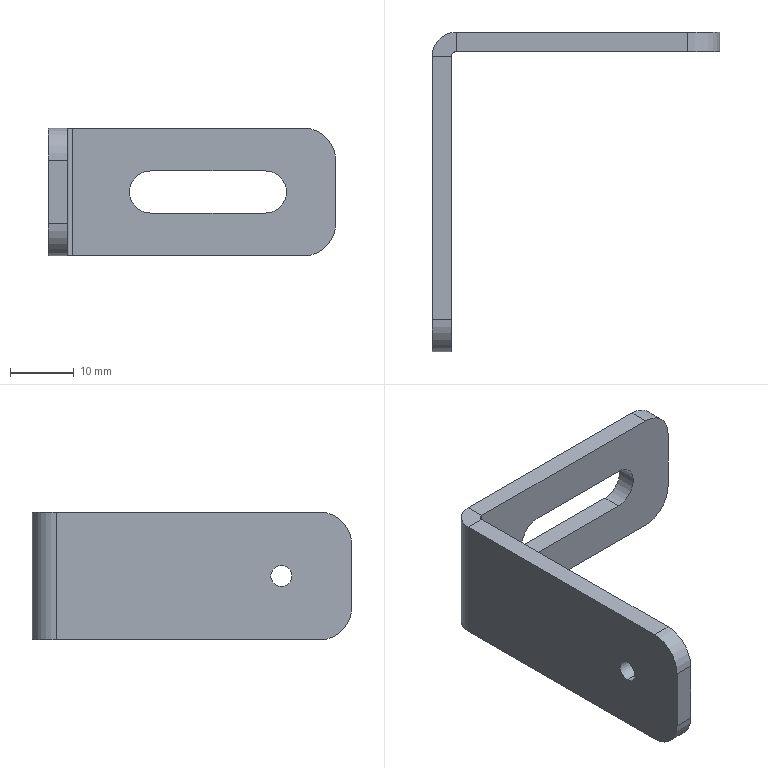Part | SolidWorks | features 3DProfileFeature 1, Fillet 1, FlatPattern 1, HoleWzd 1, ICE 1, SMBaseFlange 1, SheetMetal 1 | 1 solid | 24 faces | box 45 x 50 x 20 mm | volume 4913 mm3 | plane 14 | cylinder 10 | commonest cylinder face diameters 10 x4 3.3 x2 6.6 x2 1.473 x1 7.473 x1
STEP:
#1=CARTESIAN_POINT('',(0.,-39.,11.65));
#2=VERTEX_POINT('',#1);
#3=CARTESIAN_POINT('',(0.,-39.,8.35));
#4=VERTEX_POINT('',#3);
#5=CARTESIAN_POINT('',(0.,-39.,10.));
#6=DIRECTION('',(1.,0.,0.));
#7=DIRECTION('',(0.,0.,-1.));
#8=AXIS2_PLACEMENT_3D('',#5,#6,#7);
#9=CIRCLE('',#8,1.65);
#10=EDGE_CURVE('',#2,#4,#9,.T.);
#11=ORIENTED_EDGE('',*,*,#10,.F.);
#12=CARTESIAN_POINT('',(3.,-39.,11.65));
#13=VERTEX_POINT('',#12);
#14=CARTESIAN_POINT('',(3.,-39.,11.65));
#15=DIRECTION('',(1.,0.,0.));
#16=VECTOR('',#15,1000.);
#17=LINE('',#14,#16);
#18=EDGE_CURVE('',#2,#13,#17,.T.);
#19=ORIENTED_EDGE('',*,*,#18,.T.);
#20=CARTESIAN_POINT('',(3.,-39.,8.35));
#21=VERTEX_POINT('',#20);
#22=CARTESIAN_POINT('',(3.,-39.,10.));
#23=DIRECTION('',(1.,0.,0.));
#24=DIRECTION('',(0.,0.,-1.));
#25=AXIS2_PLACEMENT_3D('',#22,#23,#24);
#26=CIRCLE('',#25,1.65);
#27=EDGE_CURVE('',#13,#21,#26,.T.);
#28=ORIENTED_EDGE('',*,*,#27,.T.);
#29=CARTESIAN_POINT('',(3.,-39.,8.35));
#30=DIRECTION('',(1.,0.,0.));
#31=VECTOR('',#30,1000.);
#32=LINE('',#29,#31);
#33=EDGE_CURVE('',#4,#21,#32,.T.);
#34=ORIENTED_EDGE('',*,*,#33,.F.);
#35=EDGE_LOOP('',(#11,#19,#28,#34));
#36=FACE_OUTER_BOUND('',#35,.T.);
#37=CARTESIAN_POINT('',(3.,-39.,10.));
#38=DIRECTION('',(1.,0.,0.));
#39=DIRECTION('',(0.,0.,-1.));
#40=AXIS2_PLACEMENT_3D('',#37,#38,#39);
#41=CYLINDRICAL_SURFACE('',#40,1.65);
#42=ADVANCED_FACE('',(#36),#41,.F.);
#43=CARTESIAN_POINT('',(3.737,0.,20.));
#44=VERTEX_POINT('',#43);
#45=CARTESIAN_POINT('',(3.737,-3.,20.));
#46=VERTEX_POINT('',#45);
#47=CARTESIAN_POINT('',(3.737,0.,20.));
#48=DIRECTION('',(0.,-1.,0.));
#49=VECTOR('',#48,1000.);
#50=LINE('',#47,#49);
#51=EDGE_CURVE('',#44,#46,#50,.T.);
#52=ORIENTED_EDGE('',*,*,#51,.F.);
#53=CARTESIAN_POINT('',(0.,-3.737,20.));
#54=VERTEX_POINT('',#53);
#55=CARTESIAN_POINT('',(3.737,-3.737,20.));
#56=DIRECTION('',(0.,0.,-1.));
#57=DIRECTION('',(1.,0.,0.));
#58=AXIS2_PLACEMENT_3D('',#55,#56,#57);
#59=CIRCLE('',#58,3.737);
#60=EDGE_CURVE('',#54,#44,#59,.T.);
#61=ORIENTED_EDGE('',*,*,#60,.F.);
#62=CARTESIAN_POINT('',(3.,-3.737,20.));
#63=VERTEX_POINT('',#62);
#64=CARTESIAN_POINT('',(3.,-3.737,20.));
#65=DIRECTION('',(-1.,0.,0.));
#66=VECTOR('',#65,1000.);
#67=LINE('',#64,#66);
#68=EDGE_CURVE('',#63,#54,#67,.T.);
#69=ORIENTED_EDGE('',*,*,#68,.F.);
#70=CARTESIAN_POINT('',(3.737,-3.737,20.));
#71=DIRECTION('',(0.,0.,-1.));
#72=DIRECTION('',(1.,0.,0.));
#73=AXIS2_PLACEMENT_3D('',#70,#71,#72);
#74=CIRCLE('',#73,0.7366);
#75=EDGE_CURVE('',#63,#46,#74,.T.);
#76=ORIENTED_EDGE('',*,*,#75,.T.);
#77=EDGE_LOOP('',(#52,#61,#69,#76));
#78=FACE_OUTER_BOUND('',#77,.T.);
#79=CARTESIAN_POINT('',(3.737,0.,20.));
#80=DIRECTION('',(0.,0.,1.));
#81=DIRECTION('',(1.,0.,0.));
#82=AXIS2_PLACEMENT_3D('',#79,#80,#81);
#83=PLANE('',#82);
#84=ADVANCED_FACE('',(#78),#83,.T.);
#85=CARTESIAN_POINT('',(40.,-3.,20.));
#86=VERTEX_POINT('',#85);
#87=CARTESIAN_POINT('',(0.,-3.,20.));
#88=DIRECTION('',(1.,0.,0.));
#89=VECTOR('',#88,1000.);
#90=LINE('',#87,#89);
#91=EDGE_CURVE('',#46,#86,#90,.T.);
#92=ORIENTED_EDGE('',*,*,#91,.T.);
#93=CARTESIAN_POINT('',(40.,0.,20.));
#94=VERTEX_POINT('',#93);
#95=CARTESIAN_POINT('',(40.,-3.737,20.));
#96=DIRECTION('',(0.,1.,0.));
#97=VECTOR('',#96,1000.);
#98=LINE('',#95,#97);
#99=EDGE_CURVE('',#86,#94,#98,.T.);
#100=ORIENTED_EDGE('',*,*,#99,.T.);
#101=CARTESIAN_POINT('',(0.,0.,20.));
#102=DIRECTION('',(1.,0.,0.));
#103=VECTOR('',#102,1000.);
#104=LINE('',#101,#103);
#105=EDGE_CURVE('',#44,#94,#104,.T.);
#106=ORIENTED_EDGE('',*,*,#105,.F.);
#107=ORIENTED_EDGE('',*,*,#51,.T.);
#108=EDGE_LOOP('',(#92,#100,#106,#107));
#109=FACE_OUTER_BOUND('',#108,.T.);
#110=CARTESIAN_POINT('',(3.,-3.737,20.));
#111=DIRECTION('',(0.,0.,1.));
#112=DIRECTION('',(1.,0.,0.));
#113=AXIS2_PLACEMENT_3D('',#110,#111,#112);
#114=PLANE('',#113);
#115=ADVANCED_FACE('',(#109),#114,.T.);
#116=CARTESIAN_POINT('',(0.,-3.737,0.));
#117=VERTEX_POINT('',#116);
#118=CARTESIAN_POINT('',(3.,-3.737,0.));
#119=VERTEX_POINT('',#118);
#120=CARTESIAN_POINT('',(0.,-3.737,0.));
#121=DIRECTION('',(1.,0.,0.));
#122=VECTOR('',#121,1000.);
#123=LINE('',#120,#122);
#124=EDGE_CURVE('',#117,#119,#123,.T.);
#125=ORIENTED_EDGE('',*,*,#124,.F.);
#126=CARTESIAN_POINT('',(3.737,0.,0.));
#127=VERTEX_POINT('',#126);
#128=CARTESIAN_POINT('',(3.737,-3.737,0.));
#129=DIRECTION('',(0.,0.,-1.));
#130=DIRECTION('',(1.,0.,0.));
#131=AXIS2_PLACEMENT_3D('',#128,#129,#130);
#132=CIRCLE('',#131,3.737);
#133=EDGE_CURVE('',#117,#127,#132,.T.);
#134=ORIENTED_EDGE('',*,*,#133,.T.);
#135=CARTESIAN_POINT('',(3.737,-3.,0.));
#136=VERTEX_POINT('',#135);
#137=CARTESIAN_POINT('',(3.737,-3.,0.));
#138=DIRECTION('',(0.,1.,0.));
#139=VECTOR('',#138,1000.);
#140=LINE('',#137,#139);
#141=EDGE_CURVE('',#136,#127,#140,.T.);
#142=ORIENTED_EDGE('',*,*,#141,.F.);
#143=CARTESIAN_POINT('',(3.737,-3.737,0.));
#144=DIRECTION('',(0.,0.,-1.));
#145=DIRECTION('',(1.,0.,0.));
#146=AXIS2_PLACEMENT_3D('',#143,#144,#145);
#147=CIRCLE('',#146,0.7366);
#148=EDGE_CURVE('',#119,#136,#147,.T.);
#149=ORIENTED_EDGE('',*,*,#148,.F.);
#150=EDGE_LOOP('',(#125,#134,#142,#149));
#151=FACE_OUTER_BOUND('',#150,.T.);
#152=CARTESIAN_POINT('',(0.,-3.737,0.));
#153=DIRECTION('',(0.,0.,-1.));
#154=DIRECTION('',(-1.,0.,0.));
#155=AXIS2_PLACEMENT_3D('',#152,#153,#154);
#156=PLANE('',#155);
#157=ADVANCED_FACE('',(#151),#156,.T.);
#158=CARTESIAN_POINT('',(3.,-45.,0.));
#159=VERTEX_POINT('',#158);
#160=CARTESIAN_POINT('',(3.,-50.,0.));
#161=DIRECTION('',(0.,1.,0.));
#162=VECTOR('',#161,1000.);
#163=LINE('',#160,#162);
#164=EDGE_CURVE('',#159,#119,#163,.T.);
#165=ORIENTED_EDGE('',*,*,#164,.F.);
#166=CARTESIAN_POINT('',(0.,-45.,0.));
#167=VERTEX_POINT('',#166);
#168=CARTESIAN_POINT('',(3.737,-45.,0.));
#169=DIRECTION('',(-1.,0.,0.));
#170=VECTOR('',#169,1000.);
#171=LINE('',#168,#170);
#172=EDGE_CURVE('',#159,#167,#171,.T.);
#173=ORIENTED_EDGE('',*,*,#172,.T.);
#174=CARTESIAN_POINT('',(0.,-50.,0.));
#175=DIRECTION('',(0.,1.,0.));
#176=VECTOR('',#175,1000.);
#177=LINE('',#174,#176);
#178=EDGE_CURVE('',#167,#117,#177,.T.);
#179=ORIENTED_EDGE('',*,*,#178,.T.);
#180=ORIENTED_EDGE('',*,*,#124,.T.);
#181=EDGE_LOOP('',(#165,#173,#179,#180));
#182=FACE_OUTER_BOUND('',#181,.T.);
#183=CARTESIAN_POINT('',(3.737,-3.,0.));
#184=DIRECTION('',(0.,0.,-1.));
#185=DIRECTION('',(-1.,0.,0.));
#186=AXIS2_PLACEMENT_3D('',#183,#184,#185);
#187=PLANE('',#186);
#188=ADVANCED_FACE('',(#182),#187,.T.);
#189=CARTESIAN_POINT('',(16.,-3.,13.3));
#190=VERTEX_POINT('',#189);
#191=CARTESIAN_POINT('',(34.,-3.,13.3));
#192=VERTEX_POINT('',#191);
#193=CARTESIAN_POINT('',(0.,-3.,13.3));
#194=DIRECTION('',(1.,0.,0.));
#195=VECTOR('',#194,1000.);
#196=LINE('',#193,#195);
#197=EDGE_CURVE('',#190,#192,#196,.T.);
#198=ORIENTED_EDGE('',*,*,#197,.T.);
#199=CARTESIAN_POINT('',(34.,-3.,6.7));
#200=VERTEX_POINT('',#199);
#201=CARTESIAN_POINT('',(34.,-3.,10.));
#202=DIRECTION('',(0.,1.,0.));
#203=DIRECTION('',(0.,0.,1.));
#204=AXIS2_PLACEMENT_3D('',#201,#202,#203);
#205=CIRCLE('',#204,3.3);
#206=EDGE_CURVE('',#192,#200,#205,.T.);
#207=ORIENTED_EDGE('',*,*,#206,.T.);
#208=CARTESIAN_POINT('',(16.,-3.,6.7));
#209=VERTEX_POINT('',#208);
#210=CARTESIAN_POINT('',(0.,-3.,6.7));
#211=DIRECTION('',(-1.,0.,0.));
#212=VECTOR('',#211,1000.);
#213=LINE('',#210,#212);
#214=EDGE_CURVE('',#200,#209,#213,.T.);
#215=ORIENTED_EDGE('',*,*,#214,.T.);
#216=CARTESIAN_POINT('',(16.,-3.,10.));
#217=DIRECTION('',(0.,1.,0.));
#218=DIRECTION('',(0.,0.,1.));
#219=AXIS2_PLACEMENT_3D('',#216,#217,#218);
#220=CIRCLE('',#219,3.3);
#221=EDGE_CURVE('',#209,#190,#220,.T.);
#222=ORIENTED_EDGE('',*,*,#221,.T.);
#223=EDGE_LOOP('',(#198,#207,#215,#222));
#224=FACE_BOUND('',#223,.T.);
#225=CARTESIAN_POINT('',(40.,-3.,0.));
#226=VERTEX_POINT('',#225);
#227=CARTESIAN_POINT('',(0.,-3.,0.));
#228=DIRECTION('',(1.,0.,0.));
#229=VECTOR('',#228,1000.);
#230=LINE('',#227,#229);
#231=EDGE_CURVE('',#136,#226,#230,.T.);
#232=ORIENTED_EDGE('',*,*,#231,.T.);
#233=CARTESIAN_POINT('',(45.,-3.,5.));
#234=VERTEX_POINT('',#233);
#235=CARTESIAN_POINT('',(40.,-3.,5.));
#236=DIRECTION('',(0.,-1.,0.));
#237=DIRECTION('',(0.,0.,1.));
#238=AXIS2_PLACEMENT_3D('',#235,#236,#237);
#239=CIRCLE('',#238,5.);
#240=EDGE_CURVE('',#226,#234,#239,.T.);
#241=ORIENTED_EDGE('',*,*,#240,.T.);
#242=CARTESIAN_POINT('',(45.,-3.,15.));
#243=VERTEX_POINT('',#242);
#244=CARTESIAN_POINT('',(45.,-3.,20.));
#245=DIRECTION('',(0.,0.,-1.));
#246=VECTOR('',#245,1000.);
#247=LINE('',#244,#246);
#248=EDGE_CURVE('',#243,#234,#247,.T.);
#249=ORIENTED_EDGE('',*,*,#248,.F.);
#250=CARTESIAN_POINT('',(40.,-3.,15.));
#251=DIRECTION('',(0.,-1.,0.));
#252=DIRECTION('',(0.,0.,1.));
#253=AXIS2_PLACEMENT_3D('',#250,#251,#252);
#254=CIRCLE('',#253,5.);
#255=EDGE_CURVE('',#243,#86,#254,.T.);
#256=ORIENTED_EDGE('',*,*,#255,.T.);
#257=ORIENTED_EDGE('',*,*,#91,.F.);
#258=CARTESIAN_POINT('',(3.737,-3.,20.));
#259=DIRECTION('',(0.,0.,-1.));
#260=VECTOR('',#259,1000.);
#261=LINE('',#258,#260);
#262=EDGE_CURVE('',#46,#136,#261,.T.);
#263=ORIENTED_EDGE('',*,*,#262,.T.);
#264=EDGE_LOOP('',(#232,#241,#249,#256,#257,#263));
#265=FACE_OUTER_BOUND('',#264,.T.);
#266=CARTESIAN_POINT('',(0.,-3.,20.));
#267=DIRECTION('',(0.,1.,0.));
#268=DIRECTION('',(0.,0.,1.));
#269=AXIS2_PLACEMENT_3D('',#266,#267,#268);
#270=PLANE('',#269);
#271=ADVANCED_FACE('',(#224,#265),#270,.F.);
#272=ORIENTED_EDGE('',*,*,#248,.T.);
#273=CARTESIAN_POINT('',(45.,0.,5.));
#274=VERTEX_POINT('',#273);
#275=CARTESIAN_POINT('',(45.,0.,5.));
#276=DIRECTION('',(0.,1.,0.));
#277=VECTOR('',#276,1000.);
#278=LINE('',#275,#277);
#279=EDGE_CURVE('',#234,#274,#278,.T.);
#280=ORIENTED_EDGE('',*,*,#279,.T.);
#281=CARTESIAN_POINT('',(45.,0.,15.));
#282=VERTEX_POINT('',#281);
#283=CARTESIAN_POINT('',(45.,0.,20.));
#284=DIRECTION('',(0.,0.,-1.));
#285=VECTOR('',#284,1000.);
#286=LINE('',#283,#285);
#287=EDGE_CURVE('',#282,#274,#286,.T.);
#288=ORIENTED_EDGE('',*,*,#287,.F.);
#289=CARTESIAN_POINT('',(45.,0.,15.));
#290=DIRECTION('',(0.,-1.,0.));
#291=VECTOR('',#290,1000.);
#292=LINE('',#289,#291);
#293=EDGE_CURVE('',#282,#243,#292,.T.);
#294=ORIENTED_EDGE('',*,*,#293,.T.);
#295=EDGE_LOOP('',(#272,#280,#288,#294));
#296=FACE_OUTER_BOUND('',#295,.T.);
#297=CARTESIAN_POINT('',(45.,0.,20.));
#298=DIRECTION('',(1.,0.,0.));
#299=DIRECTION('',(0.,0.,-1.));
#300=AXIS2_PLACEMENT_3D('',#297,#298,#299);
#301=PLANE('',#300);
#302=ADVANCED_FACE('',(#296),#301,.T.);
#303=CARTESIAN_POINT('',(34.,0.,13.3));
#304=VERTEX_POINT('',#303);
#305=CARTESIAN_POINT('',(34.,0.,6.7));
#306=VERTEX_POINT('',#305);
#307=CARTESIAN_POINT('',(34.,0.,10.));
#308=DIRECTION('',(0.,1.,0.));
#309=DIRECTION('',(0.,0.,1.));
#310=AXIS2_PLACEMENT_3D('',#307,#308,#309);
#311=CIRCLE('',#310,3.3);
#312=EDGE_CURVE('',#304,#306,#311,.T.);
#313=ORIENTED_EDGE('',*,*,#312,.F.);
#314=CARTESIAN_POINT('',(16.,0.,13.3));
#315=VERTEX_POINT('',#314);
#316=CARTESIAN_POINT('',(34.,0.,13.3));
#317=DIRECTION('',(1.,0.,0.));
#318=VECTOR('',#317,1000.);
#319=LINE('',#316,#318);
#320=EDGE_CURVE('',#315,#304,#319,.T.);
#321=ORIENTED_EDGE('',*,*,#320,.F.);
#322=CARTESIAN_POINT('',(16.,0.,6.7));
#323=VERTEX_POINT('',#322);
#324=CARTESIAN_POINT('',(16.,0.,10.));
#325=DIRECTION('',(0.,1.,0.));
#326=DIRECTION('',(0.,0.,1.));
#327=AXIS2_PLACEMENT_3D('',#324,#325,#326);
#328=CIRCLE('',#327,3.3);
#329=EDGE_CURVE('',#323,#315,#328,.T.);
#330=ORIENTED_EDGE('',*,*,#329,.F.);
#331=CARTESIAN_POINT('',(34.,0.,6.7));
#332=DIRECTION('',(-1.,0.,0.));
#333=VECTOR('',#332,1000.);
#334=LINE('',#331,#333);
#335=EDGE_CURVE('',#306,#323,#334,.T.);
#336=ORIENTED_EDGE('',*,*,#335,.F.);
#337=EDGE_LOOP('',(#313,#321,#330,#336));
#338=FACE_BOUND('',#337,.T.);
#339=ORIENTED_EDGE('',*,*,#287,.T.);
#340=CARTESIAN_POINT('',(40.,0.,0.));
#341=VERTEX_POINT('',#340);
#342=CARTESIAN_POINT('',(40.,0.,5.));
#343=DIRECTION('',(0.,1.,0.));
#344=DIRECTION('',(0.,0.,1.));
#345=AXIS2_PLACEMENT_3D('',#342,#343,#344);
#346=CIRCLE('',#345,5.);
#347=EDGE_CURVE('',#274,#341,#346,.T.);
#348=ORIENTED_EDGE('',*,*,#347,.T.);
#349=CARTESIAN_POINT('',(0.,0.,0.));
#350=DIRECTION('',(1.,0.,0.));
#351=VECTOR('',#350,1000.);
#352=LINE('',#349,#351);
#353=EDGE_CURVE('',#127,#341,#352,.T.);
#354=ORIENTED_EDGE('',*,*,#353,.F.);
#355=CARTESIAN_POINT('',(3.737,0.,20.));
#356=DIRECTION('',(0.,0.,-1.));
#357=VECTOR('',#356,1000.);
#358=LINE('',#355,#357);
#359=EDGE_CURVE('',#44,#127,#358,.T.);
#360=ORIENTED_EDGE('',*,*,#359,.F.);
#361=ORIENTED_EDGE('',*,*,#105,.T.);
#362=CARTESIAN_POINT('',(40.,0.,15.));
#363=DIRECTION('',(0.,1.,0.));
#364=DIRECTION('',(0.,0.,1.));
#365=AXIS2_PLACEMENT_3D('',#362,#363,#364);
#366=CIRCLE('',#365,5.);
#367=EDGE_CURVE('',#94,#282,#366,.T.);
#368=ORIENTED_EDGE('',*,*,#367,.T.);
#369=EDGE_LOOP('',(#339,#348,#354,#360,#361,#368));
#370=FACE_OUTER_BOUND('',#369,.T.);
#371=CARTESIAN_POINT('',(0.,0.,20.));
#372=DIRECTION('',(0.,1.,0.));
#373=DIRECTION('',(0.,0.,1.));
#374=AXIS2_PLACEMENT_3D('',#371,#372,#373);
#375=PLANE('',#374);
#376=ADVANCED_FACE('',(#338,#370),#375,.T.);
#377=ORIENTED_EDGE('',*,*,#133,.F.);
#378=CARTESIAN_POINT('',(0.,-3.737,20.));
#379=DIRECTION('',(0.,0.,-1.));
#380=VECTOR('',#379,1000.);
#381=LINE('',#378,#380);
#382=EDGE_CURVE('',#54,#117,#381,.T.);
#383=ORIENTED_EDGE('',*,*,#382,.F.);
#384=ORIENTED_EDGE('',*,*,#60,.T.);
#385=ORIENTED_EDGE('',*,*,#359,.T.);
#386=EDGE_LOOP('',(#377,#383,#384,#385));
#387=FACE_OUTER_BOUND('',#386,.T.);
#388=CARTESIAN_POINT('',(3.737,-3.737,20.));
#389=DIRECTION('',(0.,0.,-1.));
#390=DIRECTION('',(-1.,0.,0.));
#391=AXIS2_PLACEMENT_3D('',#388,#389,#390);
#392=CYLINDRICAL_SURFACE('',#391,3.737);
#393=ADVANCED_FACE('',(#387),#392,.T.);
#394=CARTESIAN_POINT('',(0.,-39.,10.));
#395=DIRECTION('',(1.,0.,0.));
#396=DIRECTION('',(0.,0.,-1.));
#397=AXIS2_PLACEMENT_3D('',#394,#395,#396);
#398=CIRCLE('',#397,1.65);
#399=EDGE_CURVE('',#4,#2,#398,.T.);
#400=ORIENTED_EDGE('',*,*,#399,.T.);
#401=ORIENTED_EDGE('',*,*,#10,.T.);
#402=EDGE_LOOP('',(#400,#401));
#403=FACE_BOUND('',#402,.T.);
#404=ORIENTED_EDGE('',*,*,#178,.F.);
#405=CARTESIAN_POINT('',(0.,-50.,5.));
#406=VERTEX_POINT('',#405);
#407=CARTESIAN_POINT('',(0.,-45.,5.));
#408=DIRECTION('',(-1.,0.,0.));
#409=DIRECTION('',(0.,0.,1.));
#410=AXIS2_PLACEMENT_3D('',#407,#408,#409);
#411=CIRCLE('',#410,5.);
#412=EDGE_CURVE('',#167,#406,#411,.T.);
#413=ORIENTED_EDGE('',*,*,#412,.T.);
#414=CARTESIAN_POINT('',(0.,-50.,15.));
#415=VERTEX_POINT('',#414);
#416=CARTESIAN_POINT('',(0.,-50.,20.));
#417=DIRECTION('',(0.,0.,-1.));
#418=VECTOR('',#417,1000.);
#419=LINE('',#416,#418);
#420=EDGE_CURVE('',#415,#406,#419,.T.);
#421=ORIENTED_EDGE('',*,*,#420,.F.);
#422=CARTESIAN_POINT('',(0.,-45.,20.));
#423=VERTEX_POINT('',#422);
#424=CARTESIAN_POINT('',(0.,-45.,15.));
#425=DIRECTION('',(-1.,0.,0.));
#426=DIRECTION('',(0.,0.,1.));
#427=AXIS2_PLACEMENT_3D('',#424,#425,#426);
#428=CIRCLE('',#427,5.);
#429=EDGE_CURVE('',#415,#423,#428,.T.);
#430=ORIENTED_EDGE('',*,*,#429,.T.);
#431=CARTESIAN_POINT('',(0.,-50.,20.));
#432=DIRECTION('',(0.,1.,0.));
#433=VECTOR('',#432,1000.);
#434=LINE('',#431,#433);
#435=EDGE_CURVE('',#423,#54,#434,.T.);
#436=ORIENTED_EDGE('',*,*,#435,.T.);
#437=ORIENTED_EDGE('',*,*,#382,.T.);
#438=EDGE_LOOP('',(#404,#413,#421,#430,#436,#437));
#439=FACE_OUTER_BOUND('',#438,.T.);
#440=CARTESIAN_POINT('',(0.,-50.,20.));
#441=DIRECTION('',(-1.,0.,0.));
#442=DIRECTION('',(0.,0.,1.));
#443=AXIS2_PLACEMENT_3D('',#440,#441,#442);
#444=PLANE('',#443);
#445=ADVANCED_FACE('',(#403,#439),#444,.T.);
#446=ORIENTED_EDGE('',*,*,#420,.T.);
#447=CARTESIAN_POINT('',(3.,-50.,5.));
#448=VERTEX_POINT('',#447);
#449=CARTESIAN_POINT('',(3.,-50.,5.));
#450=DIRECTION('',(1.,0.,0.));
#451=VECTOR('',#450,1000.);
#452=LINE('',#449,#451);
#453=EDGE_CURVE('',#406,#448,#452,.T.);
#454=ORIENTED_EDGE('',*,*,#453,.T.);
#455=CARTESIAN_POINT('',(3.,-50.,15.));
#456=VERTEX_POINT('',#455);
#457=CARTESIAN_POINT('',(3.,-50.,20.));
#458=DIRECTION('',(0.,0.,-1.));
#459=VECTOR('',#458,1000.);
#460=LINE('',#457,#459);
#461=EDGE_CURVE('',#456,#448,#460,.T.);
#462=ORIENTED_EDGE('',*,*,#461,.F.);
#463=CARTESIAN_POINT('',(3.,-50.,15.));
#464=DIRECTION('',(-1.,0.,0.));
#465=VECTOR('',#464,1000.);
#466=LINE('',#463,#465);
#467=EDGE_CURVE('',#456,#415,#466,.T.);
#468=ORIENTED_EDGE('',*,*,#467,.T.);
#469=EDGE_LOOP('',(#446,#454,#462,#468));
#470=FACE_OUTER_BOUND('',#469,.T.);
#471=CARTESIAN_POINT('',(3.,-50.,20.));
#472=DIRECTION('',(0.,-1.,0.));
#473=DIRECTION('',(0.,0.,-1.));
#474=AXIS2_PLACEMENT_3D('',#471,#472,#473);
#475=PLANE('',#474);
#476=ADVANCED_FACE('',(#470),#475,.T.);
#477=CARTESIAN_POINT('',(3.,-39.,10.));
#478=DIRECTION('',(1.,0.,0.));
#479=DIRECTION('',(0.,0.,-1.));
#480=AXIS2_PLACEMENT_3D('',#477,#478,#479);
#481=CIRCLE('',#480,1.65);
#482=EDGE_CURVE('',#21,#13,#481,.T.);
#483=ORIENTED_EDGE('',*,*,#482,.F.);
#484=ORIENTED_EDGE('',*,*,#27,.F.);
#485=EDGE_LOOP('',(#483,#484));
#486=FACE_BOUND('',#485,.T.);
#487=ORIENTED_EDGE('',*,*,#461,.T.);
#488=CARTESIAN_POINT('',(3.,-45.,5.));
#489=DIRECTION('',(1.,0.,0.));
#490=DIRECTION('',(0.,0.,1.));
#491=AXIS2_PLACEMENT_3D('',#488,#489,#490);
#492=CIRCLE('',#491,5.);
#493=EDGE_CURVE('',#448,#159,#492,.T.);
#494=ORIENTED_EDGE('',*,*,#493,.T.);
#495=ORIENTED_EDGE('',*,*,#164,.T.);
#496=CARTESIAN_POINT('',(3.,-3.737,20.));
#497=DIRECTION('',(0.,0.,-1.));
#498=VECTOR('',#497,1000.);
#499=LINE('',#496,#498);
#500=EDGE_CURVE('',#63,#119,#499,.T.);
#501=ORIENTED_EDGE('',*,*,#500,.F.);
#502=CARTESIAN_POINT('',(3.,-45.,20.));
#503=VERTEX_POINT('',#502);
#504=CARTESIAN_POINT('',(3.,-50.,20.));
#505=DIRECTION('',(0.,1.,0.));
#506=VECTOR('',#505,1000.);
#507=LINE('',#504,#506);
#508=EDGE_CURVE('',#503,#63,#507,.T.);
#509=ORIENTED_EDGE('',*,*,#508,.F.);
#510=CARTESIAN_POINT('',(3.,-45.,15.));
#511=DIRECTION('',(1.,0.,0.));
#512=DIRECTION('',(0.,0.,1.));
#513=AXIS2_PLACEMENT_3D('',#510,#511,#512);
#514=CIRCLE('',#513,5.);
#515=EDGE_CURVE('',#503,#456,#514,.T.);
#516=ORIENTED_EDGE('',*,*,#515,.T.);
#517=EDGE_LOOP('',(#487,#494,#495,#501,#509,#516));
#518=FACE_OUTER_BOUND('',#517,.T.);
#519=CARTESIAN_POINT('',(3.,-50.,20.));
#520=DIRECTION('',(-1.,0.,0.));
#521=DIRECTION('',(0.,0.,1.));
#522=AXIS2_PLACEMENT_3D('',#519,#520,#521);
#523=PLANE('',#522);
#524=ADVANCED_FACE('',(#486,#518),#523,.F.);
#525=ORIENTED_EDGE('',*,*,#148,.T.);
#526=ORIENTED_EDGE('',*,*,#262,.F.);
#527=ORIENTED_EDGE('',*,*,#75,.F.);
#528=ORIENTED_EDGE('',*,*,#500,.T.);
#529=EDGE_LOOP('',(#525,#526,#527,#528));
#530=FACE_OUTER_BOUND('',#529,.T.);
#531=CARTESIAN_POINT('',(3.737,-3.737,20.));
#532=DIRECTION('',(0.,0.,-1.));
#533=DIRECTION('',(-1.,0.,0.));
#534=AXIS2_PLACEMENT_3D('',#531,#532,#533);
#535=CYLINDRICAL_SURFACE('',#534,0.7366);
#536=ADVANCED_FACE('',(#530),#535,.F.);
#537=ORIENTED_EDGE('',*,*,#435,.F.);
#538=CARTESIAN_POINT('',(3.737,-45.,20.));
#539=DIRECTION('',(1.,0.,0.));
#540=VECTOR('',#539,1000.);
#541=LINE('',#538,#540);
#542=EDGE_CURVE('',#423,#503,#541,.T.);
#543=ORIENTED_EDGE('',*,*,#542,.T.);
#544=ORIENTED_EDGE('',*,*,#508,.T.);
#545=ORIENTED_EDGE('',*,*,#68,.T.);
#546=EDGE_LOOP('',(#537,#543,#544,#545));
#547=FACE_OUTER_BOUND('',#546,.T.);
#548=CARTESIAN_POINT('',(3.737,-3.737,20.));
#549=DIRECTION('',(0.,0.,1.));
#550=DIRECTION('',(1.,0.,0.));
#551=AXIS2_PLACEMENT_3D('',#548,#549,#550);
#552=PLANE('',#551);
#553=ADVANCED_FACE('',(#547),#552,.T.);
#554=ORIENTED_EDGE('',*,*,#353,.T.);
#555=CARTESIAN_POINT('',(40.,-3.,0.));
#556=DIRECTION('',(0.,-1.,0.));
#557=VECTOR('',#556,1000.);
#558=LINE('',#555,#557);
#559=EDGE_CURVE('',#341,#226,#558,.T.);
#560=ORIENTED_EDGE('',*,*,#559,.T.);
#561=ORIENTED_EDGE('',*,*,#231,.F.);
#562=ORIENTED_EDGE('',*,*,#141,.T.);
#563=EDGE_LOOP('',(#554,#560,#561,#562));
#564=FACE_OUTER_BOUND('',#563,.T.);
#565=CARTESIAN_POINT('',(3.737,-3.737,0.));
#566=DIRECTION('',(0.,0.,1.));
#567=DIRECTION('',(1.,0.,0.));
#568=AXIS2_PLACEMENT_3D('',#565,#566,#567);
#569=PLANE('',#568);
#570=ADVANCED_FACE('',(#564),#569,.F.);
#571=ORIENTED_EDGE('',*,*,#493,.F.);
#572=ORIENTED_EDGE('',*,*,#453,.F.);
#573=ORIENTED_EDGE('',*,*,#412,.F.);
#574=ORIENTED_EDGE('',*,*,#172,.F.);
#575=EDGE_LOOP('',(#571,#572,#573,#574));
#576=FACE_OUTER_BOUND('',#575,.T.);
#577=CARTESIAN_POINT('',(3.737,-45.,5.));
#578=DIRECTION('',(-1.,0.,0.));
#579=DIRECTION('',(0.,0.,1.));
#580=AXIS2_PLACEMENT_3D('',#577,#578,#579);
#581=CYLINDRICAL_SURFACE('',#580,5.);
#582=ADVANCED_FACE('',(#576),#581,.T.);
#583=ORIENTED_EDGE('',*,*,#515,.F.);
#584=ORIENTED_EDGE('',*,*,#542,.F.);
#585=ORIENTED_EDGE('',*,*,#429,.F.);
#586=ORIENTED_EDGE('',*,*,#467,.F.);
#587=EDGE_LOOP('',(#583,#584,#585,#586));
#588=FACE_OUTER_BOUND('',#587,.T.);
#589=CARTESIAN_POINT('',(3.,-45.,15.));
#590=DIRECTION('',(-1.,0.,0.));
#591=DIRECTION('',(0.,0.,1.));
#592=AXIS2_PLACEMENT_3D('',#589,#590,#591);
#593=CYLINDRICAL_SURFACE('',#592,5.);
#594=ADVANCED_FACE('',(#588),#593,.T.);
#595=ORIENTED_EDGE('',*,*,#347,.F.);
#596=ORIENTED_EDGE('',*,*,#279,.F.);
#597=ORIENTED_EDGE('',*,*,#240,.F.);
#598=ORIENTED_EDGE('',*,*,#559,.F.);
#599=EDGE_LOOP('',(#595,#596,#597,#598));
#600=FACE_OUTER_BOUND('',#599,.T.);
#601=CARTESIAN_POINT('',(40.,-3.737,5.));
#602=DIRECTION('',(0.,1.,0.));
#603=DIRECTION('',(0.,0.,1.));
#604=AXIS2_PLACEMENT_3D('',#601,#602,#603);
#605=CYLINDRICAL_SURFACE('',#604,5.);
#606=ADVANCED_FACE('',(#600),#605,.T.);
#607=ORIENTED_EDGE('',*,*,#367,.F.);
#608=ORIENTED_EDGE('',*,*,#99,.F.);
#609=ORIENTED_EDGE('',*,*,#255,.F.);
#610=ORIENTED_EDGE('',*,*,#293,.F.);
#611=EDGE_LOOP('',(#607,#608,#609,#610));
#612=FACE_OUTER_BOUND('',#611,.T.);
#613=CARTESIAN_POINT('',(40.,0.,15.));
#614=DIRECTION('',(0.,-1.,0.));
#615=DIRECTION('',(0.,0.,-1.));
#616=AXIS2_PLACEMENT_3D('',#613,#614,#615);
#617=CYLINDRICAL_SURFACE('',#616,5.);
#618=ADVANCED_FACE('',(#612),#617,.T.);
#619=ORIENTED_EDGE('',*,*,#18,.F.);
#620=ORIENTED_EDGE('',*,*,#399,.F.);
#621=ORIENTED_EDGE('',*,*,#33,.T.);
#622=ORIENTED_EDGE('',*,*,#482,.T.);
#623=EDGE_LOOP('',(#619,#620,#621,#622));
#624=FACE_OUTER_BOUND('',#623,.T.);
#625=CARTESIAN_POINT('',(3.,-39.,10.));
#626=DIRECTION('',(1.,0.,0.));
#627=DIRECTION('',(0.,0.,-1.));
#628=AXIS2_PLACEMENT_3D('',#625,#626,#627);
#629=CYLINDRICAL_SURFACE('',#628,1.65);
#630=ADVANCED_FACE('',(#624),#629,.F.);
#631=CARTESIAN_POINT('',(34.,-10.,13.3));
#632=DIRECTION('',(0.,1.,0.));
#633=VECTOR('',#632,1000.);
#634=LINE('',#631,#633);
#635=EDGE_CURVE('',#192,#304,#634,.T.);
#636=ORIENTED_EDGE('',*,*,#635,.T.);
#637=ORIENTED_EDGE('',*,*,#312,.T.);
#638=CARTESIAN_POINT('',(34.,-10.,6.7));
#639=DIRECTION('',(0.,1.,0.));
#640=VECTOR('',#639,1000.);
#641=LINE('',#638,#640);
#642=EDGE_CURVE('',#200,#306,#641,.T.);
#643=ORIENTED_EDGE('',*,*,#642,.F.);
#644=ORIENTED_EDGE('',*,*,#206,.F.);
#645=EDGE_LOOP('',(#636,#637,#643,#644));
#646=FACE_OUTER_BOUND('',#645,.T.);
#647=CARTESIAN_POINT('',(34.,-10.,10.));
#648=DIRECTION('',(0.,1.,0.));
#649=DIRECTION('',(0.,0.,1.));
#650=AXIS2_PLACEMENT_3D('',#647,#648,#649);
#651=CYLINDRICAL_SURFACE('',#650,3.3);
#652=ADVANCED_FACE('',(#646),#651,.F.);
#653=CARTESIAN_POINT('',(16.,-10.,13.3));
#654=DIRECTION('',(0.,1.,0.));
#655=VECTOR('',#654,1000.);
#656=LINE('',#653,#655);
#657=EDGE_CURVE('',#190,#315,#656,.T.);
#658=ORIENTED_EDGE('',*,*,#657,.T.);
#659=ORIENTED_EDGE('',*,*,#320,.T.);
#660=ORIENTED_EDGE('',*,*,#635,.F.);
#661=ORIENTED_EDGE('',*,*,#197,.F.);
#662=EDGE_LOOP('',(#658,#659,#660,#661));
#663=FACE_OUTER_BOUND('',#662,.T.);
#664=CARTESIAN_POINT('',(34.,-10.,13.3));
#665=DIRECTION('',(0.,0.,1.));
#666=DIRECTION('',(1.,0.,0.));
#667=AXIS2_PLACEMENT_3D('',#664,#665,#666);
#668=PLANE('',#667);
#669=ADVANCED_FACE('',(#663),#668,.F.);
#670=CARTESIAN_POINT('',(16.,-10.,6.7));
#671=DIRECTION('',(0.,1.,0.));
#672=VECTOR('',#671,1000.);
#673=LINE('',#670,#672);
#674=EDGE_CURVE('',#209,#323,#673,.T.);
#675=ORIENTED_EDGE('',*,*,#674,.T.);
#676=ORIENTED_EDGE('',*,*,#329,.T.);
#677=ORIENTED_EDGE('',*,*,#657,.F.);
#678=ORIENTED_EDGE('',*,*,#221,.F.);
#679=EDGE_LOOP('',(#675,#676,#677,#678));
#680=FACE_OUTER_BOUND('',#679,.T.);
#681=CARTESIAN_POINT('',(16.,-10.,10.));
#682=DIRECTION('',(0.,1.,0.));
#683=DIRECTION('',(0.,0.,1.));
#684=AXIS2_PLACEMENT_3D('',#681,#682,#683);
#685=CYLINDRICAL_SURFACE('',#684,3.3);
#686=ADVANCED_FACE('',(#680),#685,.F.);
#687=ORIENTED_EDGE('',*,*,#642,.T.);
#688=ORIENTED_EDGE('',*,*,#335,.T.);
#689=ORIENTED_EDGE('',*,*,#674,.F.);
#690=ORIENTED_EDGE('',*,*,#214,.F.);
#691=EDGE_LOOP('',(#687,#688,#689,#690));
#692=FACE_OUTER_BOUND('',#691,.T.);
#693=CARTESIAN_POINT('',(34.,-10.,6.7));
#694=DIRECTION('',(0.,0.,-1.));
#695=DIRECTION('',(-1.,0.,0.));
#696=AXIS2_PLACEMENT_3D('',#693,#694,#695);
#697=PLANE('',#696);
#698=ADVANCED_FACE('',(#692),#697,.F.);
#699=CLOSED_SHELL('',(#42,#84,#115,#157,#188,#271,#302,#376,#393,#445,#476,#524,#536,#553,#570,#582,#594,#606,#618,#630,#652,#669,#686,#698));
#700=MANIFOLD_SOLID_BREP('',#699);
#701=CARTESIAN_POINT('',(0.,0.,0.));
#702=DIRECTION('',(0.,0.,1.));
#703=DIRECTION('',(1.,0.,0.));
#704=AXIS2_PLACEMENT_3D('',#701,#702,#703);
#705=(LENGTH_UNIT()NAMED_UNIT(*)SI_UNIT(.MILLI.,.METRE.));
#706=UNCERTAINTY_MEASURE_WITH_UNIT(LENGTH_MEASURE(0.00001),#705,'','');
#707=(NAMED_UNIT(*)PLANE_ANGLE_UNIT()SI_UNIT($,.RADIAN.));
#708=(NAMED_UNIT(*)SI_UNIT($,.STERADIAN.)SOLID_ANGLE_UNIT());
#709=(GEOMETRIC_REPRESENTATION_CONTEXT(3)GLOBAL_UNCERTAINTY_ASSIGNED_CONTEXT((#706))GLOBAL_UNIT_ASSIGNED_CONTEXT((#705,#707,#708))REPRESENTATION_CONTEXT('',''));
#710=ADVANCED_BREP_SHAPE_REPRESENTATION('',(#700,#704),#709);